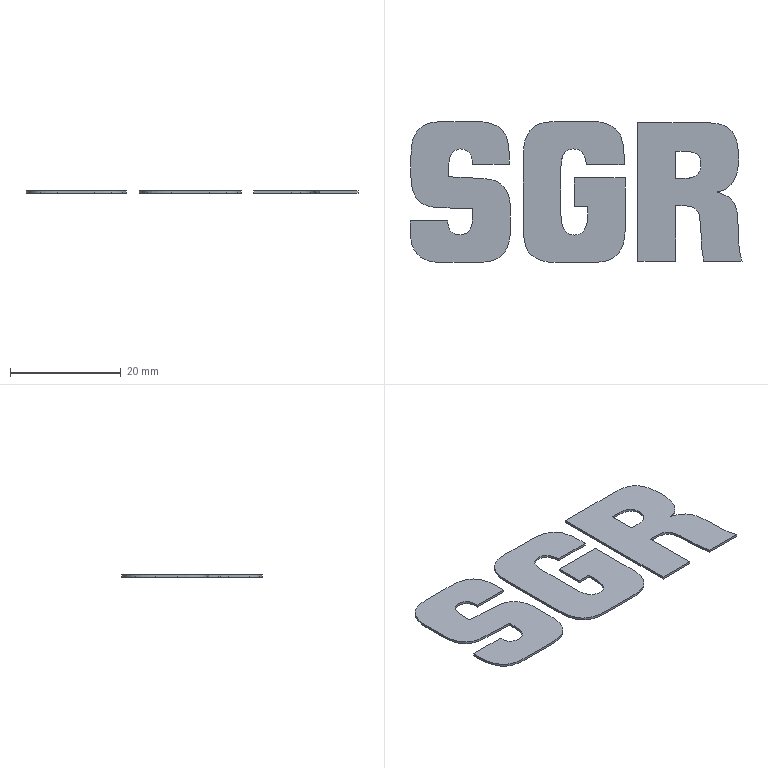Part | STEP file | S2311-1-25-SGR.stp.STEP | 3 solids | 99 faces | box 59.986 x 25.444 x 0.4165 mm | volume 459.004 mm3 | spline 60 | plane 39